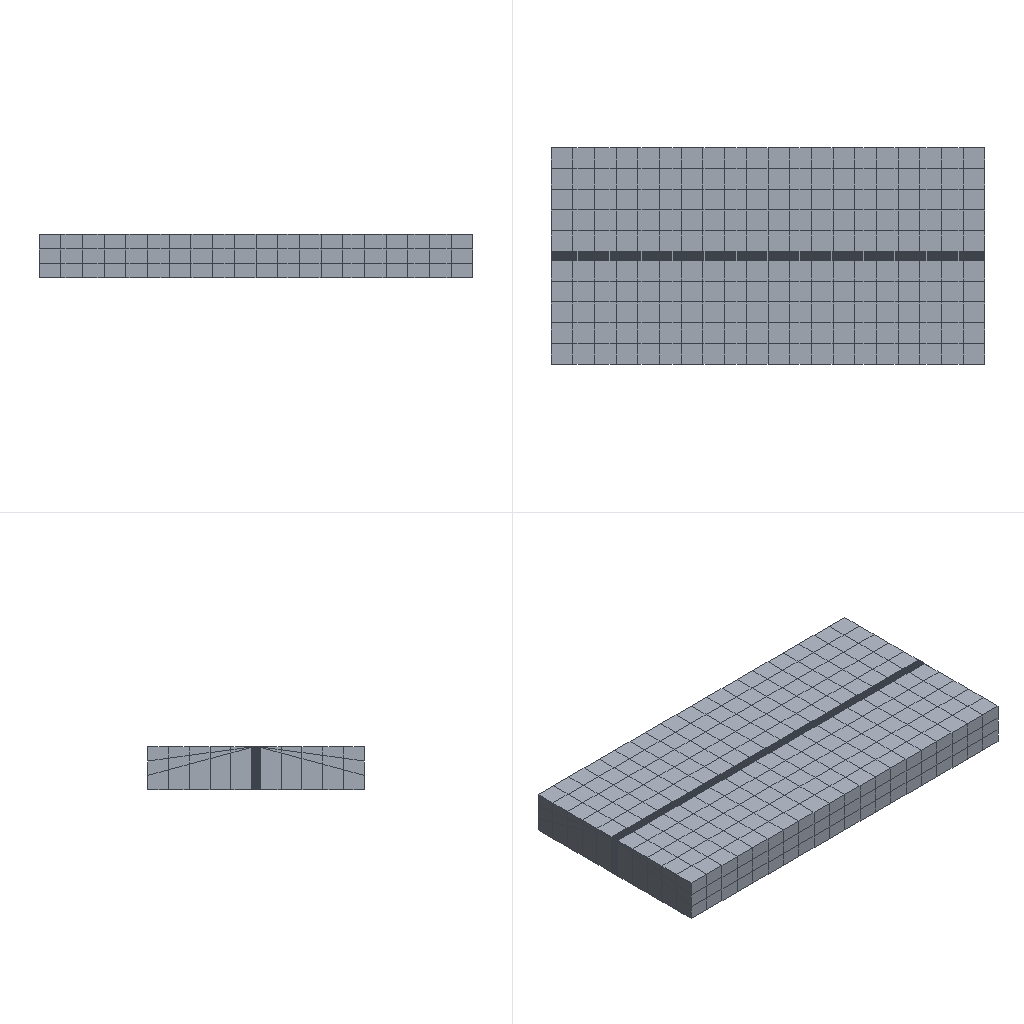Simulation study | abaqus
Set-up summary:
category,name,step,type,value,unit,region
solver,abaqus
solver,version,,,Abaqus/Standard 3DEXPERIENCE R2017x
units,not stated in the deck,,not stated
analysis,deck,,coupled temperature-displacement,coupled temperature-displacement
load_step,Step-1,Step-1,coupled temperature-displacement
load_step,requested,,,1
mesh,nodes,,,3066
mesh,elements,,,2000
element_type,C3D8RT,,solid,2000
load,load commands in deck,,count,3
bc,support commands in deck,,count,1
material,NI-TI,,in results
material,STEEL,,in results
check,setup vs results,,match,"per instance, exact: element labels, types and connectivity; labels of the nodes the elements use; coordinates of those nodes at SINGLE_PRECISION in 2 of 2 instance(s)"
Abaqus input file, long lists of numbers shortened:
*Heading
** Job name: Job-1 Model name: Job-1
** Generated by: Abaqus/CAE 2017
*Preprint, echo=NO, model=NO, history=NO, contact=NO
**
** PARTS
**
*Part, name=PART-1
*Node
      1,           0.,         -24.,   9.8
      2,           0.,         -24.,           0.
** (2602 more lines like these left out)
*Element, type=C3D8RT
   1,  116,  154,  730,  369,    1,    2,   21,   58
   2,  369,  730,  731,  370,   58,   21,   22,   57
** (1798 more lines like these left out)
*Nset, nset=SET-5, generate
    1,  2604,     1
*Elset, elset=SET-5, generate
    1,  1800,     1
** Section: Section-1-SET-5
*Solid Section, elset=SET-5, material=STEEL
,
*End Part
**
*Part, name=PART-2
*Node
      1,           0.,          -1.,  0.1
      2,           0., -0.9,  0.1
** (460 more lines like these left out)
*Element, type=C3D8RT
  1,  23,  24,  35,  34,   1,   2,  13,  12
  2,  24,  25,  36,  35,   2,   3,  14,  13
** (198 more lines like these left out)
*Nset, nset=SET-3, generate
   1,  462,    1
*Elset, elset=SET-3, generate
   1,  200,    1
** Section: Section-2-SET-3
*Solid Section, elset=SET-3, material=NI-TI
,
*End Part
**
**
** ASSEMBLY
**
*Assembly, name=Assembly
**
*Instance, name=PART-1-1, part=PART-1
*End Instance
**
*Instance, name=PART-2-1, part=PART-2
          0.,        -24.5,          10.
*End Instance
**
*Nset, nset=SET-1, instance=PART-1-1, generate
    1,  2604,     1
*Nset, nset=SET-1, instance=PART-2-1, generate
   1,  462,    1
*Elset, elset=SET-1, instance=PART-1-1, generate
    1,  1800,     1
*Elset, elset=SET-1, instance=PART-2-1, generate
   1,  200,    1
*Nset, nset=SET-2, instance=PART-1-1, generate
    1,  2604,     1
*Nset, nset=SET-2, instance=PART-2-1, generate
   1,  462,    1
*Elset, elset=SET-2, instance=PART-1-1, generate
    1,  1800,     1
*Elset, elset=SET-2, instance=PART-2-1, generate
   1,  200,    1
*Nset, nset=SET-3, instance=PART-1-1
    2,    3,    5,    6,   14,   16,   17,   19,   21,   22,   23,   24,   25,   26,   27,   28
   29,   30,   31,   32,   33,   34,   35,   36,   37,   38,   39,   59,   60,   61,   62,   63
** (39 more lines like these left out)
*Elset, elset=SET-3, instance=PART-1-1
    1,    2,    3,    4,    5,    6,    7,    8,    9,   10,   11,   12,   13,   14,   15,   16
   17,   18,   19,   20,   21,   22,   23,   24,   25,   26,   27,   28,   29,   30,   31,   32
** (36 more lines like these left out)
*Elset, elset=_JITI-SHANG_S5, internal, instance=PART-1-1
  421,  422,  423,  424,  425,  426,  427,  428,  429,  430,  431,  432,  433,  434,  435,  436
  437,  438,  439,  440,  461,  462,  463,  464,  465,  466,  467,  468,  469,  470,  471,  472
** (23 more lines like these left out)
*Elset, elset=_SURF-3_S1, internal, instance=PART-1-1
  381,  382,  383,  384,  385,  386,  387,  388,  389,  390,  391,  392,  393,  394,  395,  396
  397,  398,  399,  400, 1161, 1162, 1163, 1164, 1165, 1166, 1167, 1168, 1169, 1170, 1171, 1172
** (4 more lines like these left out)
*Elset, elset=_SURF-3_S1, internal, instance=PART-2-1, generate
 191,  200,    1
*Elset, elset=_SURF-3_S2, internal, instance=PART-1-1
    1,    2,    3,    4,    5,    6,    7,    8,    9,   10,   11,   12,   13,   14,   15,   16
   17,   18,   19,   20,  401,  402,  403,  404,  405,  406,  407,  408,  409,  410,  411,  412
** (4 more lines like these left out)
*Elset, elset=_SURF-3_S2, internal, instance=PART-2-1, generate
  1,  10,   1
*Elset, elset=_SURF-3_S3, internal, instance=PART-1-1
 1501, 1502, 1503, 1504, 1505, 1516, 1517, 1518, 1519, 1520, 1531, 1532, 1533, 1534, 1535, 1546
 1547, 1548, 1549, 1550, 1561, 1562, 1563, 1564, 1565, 1576, 1577, 1578, 1579, 1580, 1591, 1592
** (5 more lines like these left out)
*Elset, elset=_SURF-3_S3, internal, instance=PART-2-1, generate
   1,  200,    1
*Elset, elset=_SURF-3_S4, internal, instance=PART-1-1
    1,    2,    3,    4,    5,    6,    7,    8,    9,   10,   11,   12,   13,   14,   15,   16
   17,   18,   19,   20,   21,   22,   23,   24,   25,   26,   27,   28,   29,   30,   31,   32
** (33 more lines like these left out)
*Elset, elset=_SURF-3_S4, internal, instance=PART-2-1, generate
  10,  200,   10
*Elset, elset=_SURF-3_S5, internal, instance=PART-1-1
  421,  422,  423,  424,  425,  426,  427,  428,  429,  430,  431,  432,  433,  434,  435,  436
  437,  438,  439,  440,  461,  462,  463,  464,  465,  466,  467,  468,  469,  470,  471,  472
** (33 more lines like these left out)
*Elset, elset=_SURF-3_S5, internal, instance=PART-2-1, generate
   1,  200,    1
*Elset, elset=_SURF-3_S6, internal, instance=PART-1-1, generate
 1201,  1498,     3
*Elset, elset=_SURF-3_S6, internal, instance=PART-2-1, generate
   1,  191,   10
*Elset, elset=_SURF-4_S1, internal, instance=PART-1-1
  381,  382,  383,  384,  385,  386,  387,  388,  389,  390,  391,  392,  393,  394,  395,  396
  397,  398,  399,  400, 1161, 1162, 1163, 1164, 1165, 1166, 1167, 1168, 1169, 1170, 1171, 1172
** (4 more lines like these left out)
*Elset, elset=_SURF-4_S1, internal, instance=PART-2-1, generate
 191,  200,    1
*Elset, elset=_SURF-4_S2, internal, instance=PART-1-1
    1,    2,    3,    4,    5,    6,    7,    8,    9,   10,   11,   12,   13,   14,   15,   16
   17,   18,   19,   20,  401,  402,  403,  404,  405,  406,  407,  408,  409,  410,  411,  412
** (4 more lines like these left out)
*Elset, elset=_SURF-4_S2, internal, instance=PART-2-1, generate
  1,  10,   1
*Elset, elset=_SURF-4_S3, internal, instance=PART-1-1
 1501, 1502, 1503, 1504, 1505, 1516, 1517, 1518, 1519, 1520, 1531, 1532, 1533, 1534, 1535, 1546
 1547, 1548, 1549, 1550, 1561, 1562, 1563, 1564, 1565, 1576, 1577, 1578, 1579, 1580, 1591, 1592
** (5 more lines like these left out)
*Elset, elset=_SURF-4_S3, internal, instance=PART-2-1, generate
   1,  200,    1
*Elset, elset=_SURF-4_S4, internal, instance=PART-1-1
    1,    2,    3,    4,    5,    6,    7,    8,    9,   10,   11,   12,   13,   14,   15,   16
   17,   18,   19,   20,   21,   22,   23,   24,   25,   26,   27,   28,   29,   30,   31,   32
** (33 more lines like these left out)
*Elset, elset=_SURF-4_S4, internal, instance=PART-2-1, generate
  10,  200,   10
*Elset, elset=_SURF-4_S5, internal, instance=PART-1-1
  421,  422,  423,  424,  425,  426,  427,  428,  429,  430,  431,  432,  433,  434,  435,  436
  437,  438,  439,  440,  461,  462,  463,  464,  465,  466,  467,  468,  469,  470,  471,  472
** (33 more lines like these left out)
*Elset, elset=_SURF-4_S5, internal, instance=PART-2-1, generate
   1,  200,    1
*Elset, elset=_SURF-4_S6, internal, instance=PART-1-1, generate
 1201,  1498,     3
*Elset, elset=_SURF-4_S6, internal, instance=PART-2-1, generate
   1,  191,   10
*Elset, elset=_TUCENG-XIA_S5, internal, instance=PART-2-1, generate
   1,  200,    1
*Surface, type=ELEMENT, name=JITI-SHANG
_JITI-SHANG_S5, S5
*Elset, elset=_SURF-3_S2_1, internal, instance=PART-1-1
    1,    2,    3,    4,    5,    6,    7,    8,    9,   10,   11,   12,   13,   14,   15,   16
   17,   18,   19,   20,  401,  402,  403,  404,  405,  406,  407,  408,  409,  410,  411,  412
** (4 more lines like these left out)
*Elset, elset=_SURF-3_S2_1, internal, instance=PART-2-1, generate
  1,  10,   1
*Elset, elset=_SURF-3_S4_1, internal, instance=PART-1-1
    1,    2,    3,    4,    5,    6,    7,    8,    9,   10,   11,   12,   13,   14,   15,   16
   17,   18,   19,   20,   21,   22,   23,   24,   25,   26,   27,   28,   29,   30,   31,   32
** (33 more lines like these left out)
*Elset, elset=_SURF-3_S4_1, internal, instance=PART-2-1, generate
  10,  200,   10
*Elset, elset=_SURF-3_S6_1, internal, instance=PART-1-1, generate
 1201,  1498,     3
*Elset, elset=_SURF-3_S6_1, internal, instance=PART-2-1, generate
   1,  191,   10
*Elset, elset=_SURF-3_S1_1, internal, instance=PART-1-1
  381,  382,  383,  384,  385,  386,  387,  388,  389,  390,  391,  392,  393,  394,  395,  396
  397,  398,  399,  400, 1161, 1162, 1163, 1164, 1165, 1166, 1167, 1168, 1169, 1170, 1171, 1172
** (4 more lines like these left out)
*Elset, elset=_SURF-3_S1_1, internal, instance=PART-2-1, generate
 191,  200,    1
*Elset, elset=_SURF-3_S5_1, internal, instance=PART-1-1
  421,  422,  423,  424,  425,  426,  427,  428,  429,  430,  431,  432,  433,  434,  435,  436
  437,  438,  439,  440,  461,  462,  463,  464,  465,  466,  467,  468,  469,  470,  471,  472
** (33 more lines like these left out)
*Elset, elset=_SURF-3_S5_1, internal, instance=PART-2-1, generate
   1,  200,    1
*Elset, elset=_SURF-3_S3_1, internal, instance=PART-1-1
 1501, 1502, 1503, 1504, 1505, 1516, 1517, 1518, 1519, 1520, 1531, 1532, 1533, 1534, 1535, 1546
 1547, 1548, 1549, 1550, 1561, 1562, 1563, 1564, 1565, 1576, 1577, 1578, 1579, 1580, 1591, 1592
** (5 more lines like these left out)
*Elset, elset=_SURF-3_S3_1, internal, instance=PART-2-1, generate
   1,  200,    1
*Surface, type=ELEMENT, name=SURF-3
_SURF-3_S2_1, S2
_SURF-3_S4_1, S4
_SURF-3_S6_1, S6
_SURF-3_S1_1, S1
_SURF-3_S5_1, S5
_SURF-3_S3_1, S3
*Elset, elset=_SURF-4_S2_1, internal, instance=PART-1-1
    1,    2,    3,    4,    5,    6,    7,    8,    9,   10,   11,   12,   13,   14,   15,   16
   17,   18,   19,   20,  401,  402,  403,  404,  405,  406,  407,  408,  409,  410,  411,  412
** (4 more lines like these left out)
*Elset, elset=_SURF-4_S2_1, internal, instance=PART-2-1, generate
  1,  10,   1
*Elset, elset=_SURF-4_S4_1, internal, instance=PART-1-1
    1,    2,    3,    4,    5,    6,    7,    8,    9,   10,   11,   12,   13,   14,   15,   16
   17,   18,   19,   20,   21,   22,   23,   24,   25,   26,   27,   28,   29,   30,   31,   32
** (33 more lines like these left out)
*Elset, elset=_SURF-4_S4_1, internal, instance=PART-2-1, generate
  10,  200,   10
*Elset, elset=_SURF-4_S6_1, internal, instance=PART-1-1, generate
 1201,  1498,     3
*Elset, elset=_SURF-4_S6_1, internal, instance=PART-2-1, generate
   1,  191,   10
*Elset, elset=_SURF-4_S1_1, internal, instance=PART-1-1
  381,  382,  383,  384,  385,  386,  387,  388,  389,  390,  391,  392,  393,  394,  395,  396
  397,  398,  399,  400, 1161, 1162, 1163, 1164, 1165, 1166, 1167, 1168, 1169, 1170, 1171, 1172
** (4 more lines like these left out)
*Elset, elset=_SURF-4_S1_1, internal, instance=PART-2-1, generate
 191,  200,    1
*Elset, elset=_SURF-4_S5_1, internal, instance=PART-1-1
  421,  422,  423,  424,  425,  426,  427,  428,  429,  430,  431,  432,  433,  434,  435,  436
  437,  438,  439,  440,  461,  462,  463,  464,  465,  466,  467,  468,  469,  470,  471,  472
** (33 more lines like these left out)
*Elset, elset=_SURF-4_S5_1, internal, instance=PART-2-1, generate
   1,  200,    1
*Elset, elset=_SURF-4_S3_1, internal, instance=PART-1-1
 1501, 1502, 1503, 1504, 1505, 1516, 1517, 1518, 1519, 1520, 1531, 1532, 1533, 1534, 1535, 1546
 1547, 1548, 1549, 1550, 1561, 1562, 1563, 1564, 1565, 1576, 1577, 1578, 1579, 1580, 1591, 1592
** (5 more lines like these left out)
*Elset, elset=_SURF-4_S3_1, internal, instance=PART-2-1, generate
   1,  200,    1
*Surface, type=ELEMENT, name=SURF-4
_SURF-4_S2_1, S2
_SURF-4_S4_1, S4
_SURF-4_S6_1, S6
_SURF-4_S1_1, S1
_SURF-4_S5_1, S5
_SURF-4_S3_1, S3
*Surface, type=ELEMENT, name=TUCENG-XIA
_TUCENG-XIA_S5, S5
** Constraint: CONSTRAINT-1-1
*Tie, name=CONSTRAINT-1-1, adjust=yes
JITI-SHANG, TUCENG-XIA
*End Assembly
**
** MATERIALS
**
*Material, name=NI-TI
*Conductivity
10.,
*Density
 6.45e-09,
*Elastic
28000., 0.3
*Specific Heat
 3.2e+08,
*Material, name=STEEL
*Conductivity
 16.3,
*Density
 7.93e-09,
*Elastic
199000., 0.28
*Specific Heat
 5e+08,
**
** PHYSICAL CONSTANTS
**
*Physical Constants, absolute zero=-273.13, stefan boltzmann=5.67e-08
**
** BOUNDARY CONDITIONS
**
** Name: Disp-BC-1 Type: 对称/反对称/完全固定
*Boundary
SET-3, ENCASTRE
**
** PREDEFINED FIELDS
**
** Name: Field-1   Type: Temperature
*Initial Conditions, type=TEMPERATURE
SET-2, 20.
** ----------------------------------------------------------------
**
** STEP: Step-1
**
*Step, name=Step-1, nlgeom=YES
*Coupled Temperature-displacement, creep=none, deltmx=500., stabilize=0.0002, allsdtol=0.05, continue=NO
0.01, 1., 1e-05, 1.
**
** LOADS
**
** Name: BODYFLUX-1   Type: Body heat flux
*Dflux
SET-1, BFNU, 1.
**
** INTERACTIONS
**
** Interaction: SURFFILM-1
*Sfilm
SURF-3, F, 20., 10.
** Interaction: SURFRADIATE-1
*Sradiate
SURF-4, R, 20., 0.3
**
** OUTPUT REQUESTS
**
*Restart, write, frequency=0
**
** FIELD OUTPUT: F-Output-1
**
*Output, field, number interval=100
*Node Output
NT, RF, U, V
*Element Output, directions=YES
E, MISES, PE, PEEQ, S, SDEG, STATUS, TEMP
*Contact Output
CSTRESS,
**
** HISTORY OUTPUT: H-Output-1
**
*Output, history, variable=PRESELECT
*End Step
Results summary:
result,step,,partial,increments=99 time=0.99/1.0
result,analysis,,,"coupled temperature-displacement, steady state"
result,last_loadstep,,,1
result,primary field,,,"U, NT11"
result,reaction total,,FX,0.0,model units
result,reaction total,,FY,0.0,model units
result,reaction total,,FZ,0.0,model units